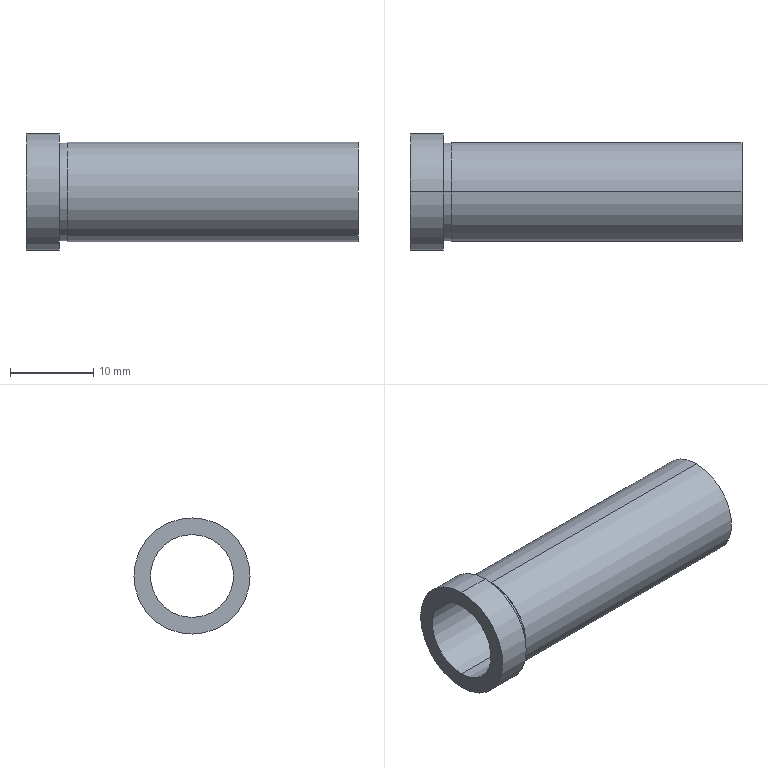Part | SolidWorks | features RefAxis 3, 3DProfileFeature 1, Revolution 1 | 1 solid | 12 faces | box 40 x 14 x 14 mm | volume 1542 mm3 | cylinder 8 | plane 4 | commonest cylinder face diameters 10 x2 11.8 x2 12 x2 14 x2
STEP:
#1=CARTESIAN_POINT('',(-15.,0.,5.9));
#2=VERTEX_POINT('',#1);
#3=CARTESIAN_POINT('',(-15.,0.,-5.9));
#4=VERTEX_POINT('',#3);
#5=CARTESIAN_POINT('',(-15.,0.,0.));
#6=DIRECTION('',(-1.,0.,0.));
#7=DIRECTION('',(0.,0.,1.));
#8=AXIS2_PLACEMENT_3D('',#5,#6,#7);
#9=CIRCLE('',#8,5.9);
#10=EDGE_CURVE('',#2,#4,#9,.T.);
#11=ORIENTED_EDGE('',*,*,#10,.T.);
#12=CARTESIAN_POINT('',(-16.,0.,-5.9));
#13=VERTEX_POINT('',#12);
#14=CARTESIAN_POINT('',(20.,0.,-5.9));
#15=DIRECTION('',(-1.,0.,0.));
#16=VECTOR('',#15,1000.);
#17=LINE('',#14,#16);
#18=EDGE_CURVE('',#4,#13,#17,.T.);
#19=ORIENTED_EDGE('',*,*,#18,.T.);
#20=CARTESIAN_POINT('',(-16.,0.,5.9));
#21=VERTEX_POINT('',#20);
#22=CARTESIAN_POINT('',(-16.,0.,0.));
#23=DIRECTION('',(-1.,0.,0.));
#24=DIRECTION('',(0.,0.,1.));
#25=AXIS2_PLACEMENT_3D('',#22,#23,#24);
#26=CIRCLE('',#25,5.9);
#27=EDGE_CURVE('',#21,#13,#26,.T.);
#28=ORIENTED_EDGE('',*,*,#27,.F.);
#29=CARTESIAN_POINT('',(20.,0.,5.9));
#30=DIRECTION('',(-1.,0.,0.));
#31=VECTOR('',#30,1000.);
#32=LINE('',#29,#31);
#33=EDGE_CURVE('',#2,#21,#32,.T.);
#34=ORIENTED_EDGE('',*,*,#33,.F.);
#35=EDGE_LOOP('',(#11,#19,#28,#34));
#36=FACE_OUTER_BOUND('',#35,.T.);
#37=CARTESIAN_POINT('',(20.,0.,0.));
#38=DIRECTION('',(-1.,0.,0.));
#39=DIRECTION('',(0.,0.,1.));
#40=AXIS2_PLACEMENT_3D('',#37,#38,#39);
#41=CYLINDRICAL_SURFACE('',#40,5.9);
#42=ADVANCED_FACE('',(#36),#41,.T.);
#43=CARTESIAN_POINT('',(20.,0.,6.));
#44=VERTEX_POINT('',#43);
#45=CARTESIAN_POINT('',(20.,0.,-6.));
#46=VERTEX_POINT('',#45);
#47=CARTESIAN_POINT('',(20.,0.,0.));
#48=DIRECTION('',(-1.,0.,0.));
#49=DIRECTION('',(0.,0.,1.));
#50=AXIS2_PLACEMENT_3D('',#47,#48,#49);
#51=CIRCLE('',#50,6.);
#52=EDGE_CURVE('',#44,#46,#51,.T.);
#53=ORIENTED_EDGE('',*,*,#52,.T.);
#54=CARTESIAN_POINT('',(-15.,0.,-6.));
#55=VERTEX_POINT('',#54);
#56=CARTESIAN_POINT('',(20.,0.,-6.));
#57=DIRECTION('',(-1.,0.,0.));
#58=VECTOR('',#57,1000.);
#59=LINE('',#56,#58);
#60=EDGE_CURVE('',#46,#55,#59,.T.);
#61=ORIENTED_EDGE('',*,*,#60,.T.);
#62=CARTESIAN_POINT('',(-15.,0.,6.));
#63=VERTEX_POINT('',#62);
#64=CARTESIAN_POINT('',(-15.,0.,0.));
#65=DIRECTION('',(-1.,0.,0.));
#66=DIRECTION('',(0.,0.,1.));
#67=AXIS2_PLACEMENT_3D('',#64,#65,#66);
#68=CIRCLE('',#67,6.);
#69=EDGE_CURVE('',#63,#55,#68,.T.);
#70=ORIENTED_EDGE('',*,*,#69,.F.);
#71=CARTESIAN_POINT('',(20.,0.,6.));
#72=DIRECTION('',(-1.,0.,0.));
#73=VECTOR('',#72,1000.);
#74=LINE('',#71,#73);
#75=EDGE_CURVE('',#44,#63,#74,.T.);
#76=ORIENTED_EDGE('',*,*,#75,.F.);
#77=EDGE_LOOP('',(#53,#61,#70,#76));
#78=FACE_OUTER_BOUND('',#77,.T.);
#79=CARTESIAN_POINT('',(20.,0.,0.));
#80=DIRECTION('',(-1.,0.,0.));
#81=DIRECTION('',(0.,0.,1.));
#82=AXIS2_PLACEMENT_3D('',#79,#80,#81);
#83=CYLINDRICAL_SURFACE('',#82,6.);
#84=ADVANCED_FACE('',(#78),#83,.T.);
#85=CARTESIAN_POINT('',(20.,0.,-5.));
#86=VERTEX_POINT('',#85);
#87=CARTESIAN_POINT('',(20.,0.,5.));
#88=VERTEX_POINT('',#87);
#89=CARTESIAN_POINT('',(20.,0.,0.));
#90=DIRECTION('',(-1.,0.,0.));
#91=DIRECTION('',(0.,0.,1.));
#92=AXIS2_PLACEMENT_3D('',#89,#90,#91);
#93=CIRCLE('',#92,5.);
#94=EDGE_CURVE('',#86,#88,#93,.T.);
#95=ORIENTED_EDGE('',*,*,#94,.F.);
#96=CARTESIAN_POINT('',(-20.,0.,-5.));
#97=VERTEX_POINT('',#96);
#98=CARTESIAN_POINT('',(20.,0.,-5.));
#99=DIRECTION('',(-1.,0.,0.));
#100=VECTOR('',#99,1000.);
#101=LINE('',#98,#100);
#102=EDGE_CURVE('',#86,#97,#101,.T.);
#103=ORIENTED_EDGE('',*,*,#102,.T.);
#104=CARTESIAN_POINT('',(-20.,0.,5.));
#105=VERTEX_POINT('',#104);
#106=CARTESIAN_POINT('',(-20.,0.,0.));
#107=DIRECTION('',(-1.,0.,0.));
#108=DIRECTION('',(0.,0.,1.));
#109=AXIS2_PLACEMENT_3D('',#106,#107,#108);
#110=CIRCLE('',#109,5.);
#111=EDGE_CURVE('',#97,#105,#110,.T.);
#112=ORIENTED_EDGE('',*,*,#111,.T.);
#113=CARTESIAN_POINT('',(20.,0.,5.));
#114=DIRECTION('',(-1.,0.,0.));
#115=VECTOR('',#114,1000.);
#116=LINE('',#113,#115);
#117=EDGE_CURVE('',#88,#105,#116,.T.);
#118=ORIENTED_EDGE('',*,*,#117,.F.);
#119=EDGE_LOOP('',(#95,#103,#112,#118));
#120=FACE_OUTER_BOUND('',#119,.T.);
#121=CARTESIAN_POINT('',(20.,0.,0.));
#122=DIRECTION('',(-1.,0.,0.));
#123=DIRECTION('',(0.,0.,1.));
#124=AXIS2_PLACEMENT_3D('',#121,#122,#123);
#125=CYLINDRICAL_SURFACE('',#124,5.);
#126=ADVANCED_FACE('',(#120),#125,.F.);
#127=CARTESIAN_POINT('',(-16.,0.,7.));
#128=VERTEX_POINT('',#127);
#129=CARTESIAN_POINT('',(-16.,0.,-7.));
#130=VERTEX_POINT('',#129);
#131=CARTESIAN_POINT('',(-16.,0.,0.));
#132=DIRECTION('',(-1.,0.,0.));
#133=DIRECTION('',(0.,0.,1.));
#134=AXIS2_PLACEMENT_3D('',#131,#132,#133);
#135=CIRCLE('',#134,7.);
#136=EDGE_CURVE('',#128,#130,#135,.T.);
#137=ORIENTED_EDGE('',*,*,#136,.T.);
#138=CARTESIAN_POINT('',(-20.,0.,-7.));
#139=VERTEX_POINT('',#138);
#140=CARTESIAN_POINT('',(20.,0.,-7.));
#141=DIRECTION('',(-1.,0.,0.));
#142=VECTOR('',#141,1000.);
#143=LINE('',#140,#142);
#144=EDGE_CURVE('',#130,#139,#143,.T.);
#145=ORIENTED_EDGE('',*,*,#144,.T.);
#146=CARTESIAN_POINT('',(-20.,0.,7.));
#147=VERTEX_POINT('',#146);
#148=CARTESIAN_POINT('',(-20.,0.,0.));
#149=DIRECTION('',(-1.,0.,0.));
#150=DIRECTION('',(0.,0.,1.));
#151=AXIS2_PLACEMENT_3D('',#148,#149,#150);
#152=CIRCLE('',#151,7.);
#153=EDGE_CURVE('',#147,#139,#152,.T.);
#154=ORIENTED_EDGE('',*,*,#153,.F.);
#155=CARTESIAN_POINT('',(20.,0.,7.));
#156=DIRECTION('',(-1.,0.,0.));
#157=VECTOR('',#156,1000.);
#158=LINE('',#155,#157);
#159=EDGE_CURVE('',#128,#147,#158,.T.);
#160=ORIENTED_EDGE('',*,*,#159,.F.);
#161=EDGE_LOOP('',(#137,#145,#154,#160));
#162=FACE_OUTER_BOUND('',#161,.T.);
#163=CARTESIAN_POINT('',(20.,0.,0.));
#164=DIRECTION('',(-1.,0.,0.));
#165=DIRECTION('',(0.,0.,1.));
#166=AXIS2_PLACEMENT_3D('',#163,#164,#165);
#167=CYLINDRICAL_SURFACE('',#166,7.);
#168=ADVANCED_FACE('',(#162),#167,.T.);
#169=ORIENTED_EDGE('',*,*,#144,.F.);
#170=CARTESIAN_POINT('',(-16.,0.,0.));
#171=DIRECTION('',(-1.,0.,0.));
#172=DIRECTION('',(0.,0.,1.));
#173=AXIS2_PLACEMENT_3D('',#170,#171,#172);
#174=CIRCLE('',#173,7.);
#175=EDGE_CURVE('',#130,#128,#174,.T.);
#176=ORIENTED_EDGE('',*,*,#175,.T.);
#177=ORIENTED_EDGE('',*,*,#159,.T.);
#178=CARTESIAN_POINT('',(-20.,0.,0.));
#179=DIRECTION('',(-1.,0.,0.));
#180=DIRECTION('',(0.,0.,1.));
#181=AXIS2_PLACEMENT_3D('',#178,#179,#180);
#182=CIRCLE('',#181,7.);
#183=EDGE_CURVE('',#139,#147,#182,.T.);
#184=ORIENTED_EDGE('',*,*,#183,.F.);
#185=EDGE_LOOP('',(#169,#176,#177,#184));
#186=FACE_OUTER_BOUND('',#185,.T.);
#187=CARTESIAN_POINT('',(20.,0.,0.));
#188=DIRECTION('',(-1.,0.,0.));
#189=DIRECTION('',(0.,0.,1.));
#190=AXIS2_PLACEMENT_3D('',#187,#188,#189);
#191=CYLINDRICAL_SURFACE('',#190,7.);
#192=ADVANCED_FACE('',(#186),#191,.T.);
#193=CARTESIAN_POINT('',(-20.,0.,0.));
#194=DIRECTION('',(-1.,0.,0.));
#195=DIRECTION('',(0.,0.,1.));
#196=AXIS2_PLACEMENT_3D('',#193,#194,#195);
#197=CIRCLE('',#196,5.);
#198=EDGE_CURVE('',#105,#97,#197,.T.);
#199=ORIENTED_EDGE('',*,*,#198,.F.);
#200=ORIENTED_EDGE('',*,*,#111,.F.);
#201=EDGE_LOOP('',(#199,#200));
#202=FACE_BOUND('',#201,.T.);
#203=ORIENTED_EDGE('',*,*,#153,.T.);
#204=ORIENTED_EDGE('',*,*,#183,.T.);
#205=EDGE_LOOP('',(#203,#204));
#206=FACE_OUTER_BOUND('',#205,.T.);
#207=CARTESIAN_POINT('',(-20.,7.,0.));
#208=DIRECTION('',(1.,0.,0.));
#209=DIRECTION('',(0.,0.,-1.));
#210=AXIS2_PLACEMENT_3D('',#207,#208,#209);
#211=PLANE('',#210);
#212=ADVANCED_FACE('',(#202,#206),#211,.F.);
#213=ORIENTED_EDGE('',*,*,#102,.F.);
#214=CARTESIAN_POINT('',(20.,0.,0.));
#215=DIRECTION('',(-1.,0.,0.));
#216=DIRECTION('',(0.,0.,1.));
#217=AXIS2_PLACEMENT_3D('',#214,#215,#216);
#218=CIRCLE('',#217,5.);
#219=EDGE_CURVE('',#88,#86,#218,.T.);
#220=ORIENTED_EDGE('',*,*,#219,.F.);
#221=ORIENTED_EDGE('',*,*,#117,.T.);
#222=ORIENTED_EDGE('',*,*,#198,.T.);
#223=EDGE_LOOP('',(#213,#220,#221,#222));
#224=FACE_OUTER_BOUND('',#223,.T.);
#225=CARTESIAN_POINT('',(20.,0.,0.));
#226=DIRECTION('',(-1.,0.,0.));
#227=DIRECTION('',(0.,0.,1.));
#228=AXIS2_PLACEMENT_3D('',#225,#226,#227);
#229=CYLINDRICAL_SURFACE('',#228,5.);
#230=ADVANCED_FACE('',(#224),#229,.F.);
#231=ORIENTED_EDGE('',*,*,#52,.F.);
#232=CARTESIAN_POINT('',(20.,0.,0.));
#233=DIRECTION('',(-1.,0.,0.));
#234=DIRECTION('',(0.,0.,1.));
#235=AXIS2_PLACEMENT_3D('',#232,#233,#234);
#236=CIRCLE('',#235,6.);
#237=EDGE_CURVE('',#46,#44,#236,.T.);
#238=ORIENTED_EDGE('',*,*,#237,.F.);
#239=EDGE_LOOP('',(#231,#238));
#240=FACE_OUTER_BOUND('',#239,.T.);
#241=ORIENTED_EDGE('',*,*,#219,.T.);
#242=ORIENTED_EDGE('',*,*,#94,.T.);
#243=EDGE_LOOP('',(#241,#242));
#244=FACE_BOUND('',#243,.T.);
#245=CARTESIAN_POINT('',(20.,5.,0.));
#246=DIRECTION('',(-1.,0.,0.));
#247=DIRECTION('',(0.,0.,1.));
#248=AXIS2_PLACEMENT_3D('',#245,#246,#247);
#249=PLANE('',#248);
#250=ADVANCED_FACE('',(#240,#244),#249,.F.);
#251=ORIENTED_EDGE('',*,*,#60,.F.);
#252=ORIENTED_EDGE('',*,*,#237,.T.);
#253=ORIENTED_EDGE('',*,*,#75,.T.);
#254=CARTESIAN_POINT('',(-15.,0.,0.));
#255=DIRECTION('',(-1.,0.,0.));
#256=DIRECTION('',(0.,0.,1.));
#257=AXIS2_PLACEMENT_3D('',#254,#255,#256);
#258=CIRCLE('',#257,6.);
#259=EDGE_CURVE('',#55,#63,#258,.T.);
#260=ORIENTED_EDGE('',*,*,#259,.F.);
#261=EDGE_LOOP('',(#251,#252,#253,#260));
#262=FACE_OUTER_BOUND('',#261,.T.);
#263=CARTESIAN_POINT('',(20.,0.,0.));
#264=DIRECTION('',(-1.,0.,0.));
#265=DIRECTION('',(0.,0.,1.));
#266=AXIS2_PLACEMENT_3D('',#263,#264,#265);
#267=CYLINDRICAL_SURFACE('',#266,6.);
#268=ADVANCED_FACE('',(#262),#267,.T.);
#269=ORIENTED_EDGE('',*,*,#10,.F.);
#270=CARTESIAN_POINT('',(-15.,0.,0.));
#271=DIRECTION('',(-1.,0.,0.));
#272=DIRECTION('',(0.,0.,1.));
#273=AXIS2_PLACEMENT_3D('',#270,#271,#272);
#274=CIRCLE('',#273,5.9);
#275=EDGE_CURVE('',#4,#2,#274,.T.);
#276=ORIENTED_EDGE('',*,*,#275,.F.);
#277=EDGE_LOOP('',(#269,#276));
#278=FACE_BOUND('',#277,.T.);
#279=ORIENTED_EDGE('',*,*,#69,.T.);
#280=ORIENTED_EDGE('',*,*,#259,.T.);
#281=EDGE_LOOP('',(#279,#280));
#282=FACE_OUTER_BOUND('',#281,.T.);
#283=CARTESIAN_POINT('',(-15.,6.,0.));
#284=DIRECTION('',(1.,0.,0.));
#285=DIRECTION('',(0.,0.,-1.));
#286=AXIS2_PLACEMENT_3D('',#283,#284,#285);
#287=PLANE('',#286);
#288=ADVANCED_FACE('',(#278,#282),#287,.F.);
#289=ORIENTED_EDGE('',*,*,#18,.F.);
#290=ORIENTED_EDGE('',*,*,#275,.T.);
#291=ORIENTED_EDGE('',*,*,#33,.T.);
#292=CARTESIAN_POINT('',(-16.,0.,0.));
#293=DIRECTION('',(-1.,0.,0.));
#294=DIRECTION('',(0.,0.,1.));
#295=AXIS2_PLACEMENT_3D('',#292,#293,#294);
#296=CIRCLE('',#295,5.9);
#297=EDGE_CURVE('',#13,#21,#296,.T.);
#298=ORIENTED_EDGE('',*,*,#297,.F.);
#299=EDGE_LOOP('',(#289,#290,#291,#298));
#300=FACE_OUTER_BOUND('',#299,.T.);
#301=CARTESIAN_POINT('',(20.,0.,0.));
#302=DIRECTION('',(-1.,0.,0.));
#303=DIRECTION('',(0.,0.,1.));
#304=AXIS2_PLACEMENT_3D('',#301,#302,#303);
#305=CYLINDRICAL_SURFACE('',#304,5.9);
#306=ADVANCED_FACE('',(#300),#305,.T.);
#307=ORIENTED_EDGE('',*,*,#136,.F.);
#308=ORIENTED_EDGE('',*,*,#175,.F.);
#309=EDGE_LOOP('',(#307,#308));
#310=FACE_OUTER_BOUND('',#309,.T.);
#311=ORIENTED_EDGE('',*,*,#27,.T.);
#312=ORIENTED_EDGE('',*,*,#297,.T.);
#313=EDGE_LOOP('',(#311,#312));
#314=FACE_BOUND('',#313,.T.);
#315=CARTESIAN_POINT('',(-16.,5.9,0.));
#316=DIRECTION('',(-1.,0.,0.));
#317=DIRECTION('',(0.,0.,1.));
#318=AXIS2_PLACEMENT_3D('',#315,#316,#317);
#319=PLANE('',#318);
#320=ADVANCED_FACE('',(#310,#314),#319,.F.);
#321=CLOSED_SHELL('',(#42,#84,#126,#168,#192,#212,#230,#250,#268,#288,#306,#320));
#322=MANIFOLD_SOLID_BREP('',#321);
#323=CARTESIAN_POINT('',(0.,0.,0.));
#324=DIRECTION('',(0.,0.,1.));
#325=DIRECTION('',(1.,0.,0.));
#326=AXIS2_PLACEMENT_3D('',#323,#324,#325);
#327=(LENGTH_UNIT()NAMED_UNIT(*)SI_UNIT(.MILLI.,.METRE.));
#328=UNCERTAINTY_MEASURE_WITH_UNIT(LENGTH_MEASURE(0.00001),#327,'','');
#329=(NAMED_UNIT(*)PLANE_ANGLE_UNIT()SI_UNIT($,.RADIAN.));
#330=(NAMED_UNIT(*)SI_UNIT($,.STERADIAN.)SOLID_ANGLE_UNIT());
#331=(GEOMETRIC_REPRESENTATION_CONTEXT(3)GLOBAL_UNCERTAINTY_ASSIGNED_CONTEXT((#328))GLOBAL_UNIT_ASSIGNED_CONTEXT((#327,#329,#330))REPRESENTATION_CONTEXT('',''));
#332=ADVANCED_BREP_SHAPE_REPRESENTATION('',(#322,#326),#331);